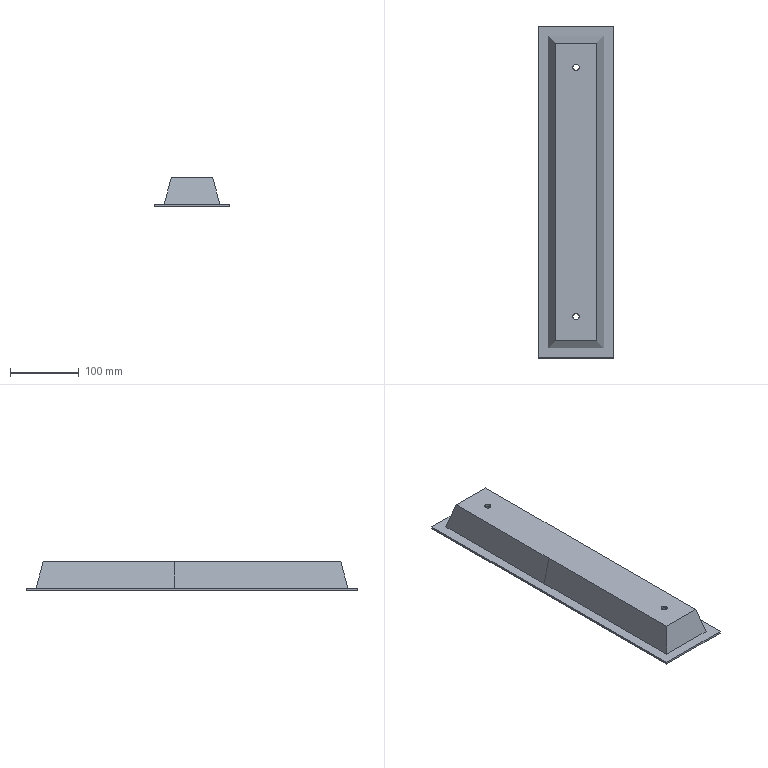Part | NX | features BREP 1 | 1 solid | 28 faces | box 110 x 481.5 x 42.13 mm | volume 250007 mm3 | plane 20 | cylinder 8 | commonest cylinder face diameters 9 x8
STEP:
#1=CARTESIAN_POINT('',(1224.372,-309.5,70.005));
#2=VERTEX_POINT('',#1);
#3=CARTESIAN_POINT('',(1224.372,-309.5,67.005));
#4=VERTEX_POINT('',#3);
#5=CARTESIAN_POINT('',(1224.372,-309.5,68.505));
#6=DIRECTION('',(0.,0.,-1.));
#7=VECTOR('',#6,1000.);
#8=LINE('',#5,#7);
#9=EDGE_CURVE('',#2,#4,#8,.T.);
#10=ORIENTED_EDGE('',*,*,#9,.T.);
#11=CARTESIAN_POINT('',(1224.372,-791.,67.005));
#12=VERTEX_POINT('',#11);
#13=CARTESIAN_POINT('',(1224.372,-550.25,67.005));
#14=DIRECTION('',(0.,1.,0.));
#15=VECTOR('',#14,1000.);
#16=LINE('',#13,#15);
#17=EDGE_CURVE('',#12,#4,#16,.T.);
#18=ORIENTED_EDGE('',*,*,#17,.F.);
#19=CARTESIAN_POINT('',(1224.372,-791.,70.005));
#20=VERTEX_POINT('',#19);
#21=CARTESIAN_POINT('',(1224.372,-791.,68.505));
#22=DIRECTION('',(0.,0.,-1.));
#23=VECTOR('',#22,1000.);
#24=LINE('',#21,#23);
#25=EDGE_CURVE('',#20,#12,#24,.T.);
#26=ORIENTED_EDGE('',*,*,#25,.F.);
#27=CARTESIAN_POINT('',(1224.372,-550.25,70.005));
#28=DIRECTION('',(0.,1.,0.));
#29=VECTOR('',#28,1000.);
#30=LINE('',#27,#29);
#31=EDGE_CURVE('',#20,#2,#30,.T.);
#32=ORIENTED_EDGE('',*,*,#31,.T.);
#33=EDGE_LOOP('',(#10,#18,#26,#32));
#34=FACE_BOUND('',#33,.T.);
#35=CARTESIAN_POINT('',(1224.372,-550.25,70.005));
#36=DIRECTION('',(1.,0.,0.));
#37=DIRECTION('',(0.,0.,-1.));
#38=AXIS2_PLACEMENT_3D('',#35,#36,#37);
#39=PLANE('',#38);
#40=ADVANCED_FACE('',(#34),#39,.F.);
#41=CARTESIAN_POINT('',(1334.372,-791.,70.005));
#42=VERTEX_POINT('',#41);
#43=CARTESIAN_POINT('',(1279.372,-791.,70.005));
#44=DIRECTION('',(1.,0.,0.));
#45=VECTOR('',#44,1000.);
#46=LINE('',#43,#45);
#47=EDGE_CURVE('',#20,#42,#46,.T.);
#48=ORIENTED_EDGE('',*,*,#47,.F.);
#49=ORIENTED_EDGE('',*,*,#25,.T.);
#50=CARTESIAN_POINT('',(1334.372,-791.,67.005));
#51=VERTEX_POINT('',#50);
#52=CARTESIAN_POINT('',(1279.372,-791.,67.005));
#53=DIRECTION('',(1.,0.,0.));
#54=VECTOR('',#53,1000.);
#55=LINE('',#52,#54);
#56=EDGE_CURVE('',#12,#51,#55,.T.);
#57=ORIENTED_EDGE('',*,*,#56,.T.);
#58=CARTESIAN_POINT('',(1334.372,-791.,68.505));
#59=DIRECTION('',(0.,0.,-1.));
#60=VECTOR('',#59,1000.);
#61=LINE('',#58,#60);
#62=EDGE_CURVE('',#42,#51,#61,.T.);
#63=ORIENTED_EDGE('',*,*,#62,.F.);
#64=EDGE_LOOP('',(#48,#49,#57,#63));
#65=FACE_BOUND('',#64,.T.);
#66=CARTESIAN_POINT('',(1279.372,-791.,70.005));
#67=DIRECTION('',(0.,1.,0.));
#68=DIRECTION('',(1.,0.,0.));
#69=AXIS2_PLACEMENT_3D('',#66,#67,#68);
#70=PLANE('',#69);
#71=ADVANCED_FACE('',(#65),#70,.F.);
#72=CARTESIAN_POINT('',(1334.372,-309.5,70.005));
#73=VERTEX_POINT('',#72);
#74=CARTESIAN_POINT('',(1334.372,-550.25,70.005));
#75=DIRECTION('',(0.,-1.,0.));
#76=VECTOR('',#75,1000.);
#77=LINE('',#74,#76);
#78=EDGE_CURVE('',#73,#42,#77,.T.);
#79=ORIENTED_EDGE('',*,*,#78,.T.);
#80=ORIENTED_EDGE('',*,*,#62,.T.);
#81=CARTESIAN_POINT('',(1334.372,-309.5,67.005));
#82=VERTEX_POINT('',#81);
#83=CARTESIAN_POINT('',(1334.372,-550.25,67.005));
#84=DIRECTION('',(0.,1.,0.));
#85=VECTOR('',#84,1000.);
#86=LINE('',#83,#85);
#87=EDGE_CURVE('',#51,#82,#86,.T.);
#88=ORIENTED_EDGE('',*,*,#87,.T.);
#89=CARTESIAN_POINT('',(1334.372,-309.5,68.505));
#90=DIRECTION('',(0.,0.,-1.));
#91=VECTOR('',#90,1000.);
#92=LINE('',#89,#91);
#93=EDGE_CURVE('',#73,#82,#92,.T.);
#94=ORIENTED_EDGE('',*,*,#93,.F.);
#95=EDGE_LOOP('',(#79,#80,#88,#94));
#96=FACE_BOUND('',#95,.T.);
#97=CARTESIAN_POINT('',(1334.372,-550.25,70.005));
#98=DIRECTION('',(-1.,0.,0.));
#99=DIRECTION('',(0.,0.,-1.));
#100=AXIS2_PLACEMENT_3D('',#97,#98,#99);
#101=PLANE('',#100);
#102=ADVANCED_FACE('',(#96),#101,.F.);
#103=CARTESIAN_POINT('',(1279.372,-309.5,70.005));
#104=DIRECTION('',(1.,0.,0.));
#105=VECTOR('',#104,1000.);
#106=LINE('',#103,#105);
#107=EDGE_CURVE('',#2,#73,#106,.T.);
#108=ORIENTED_EDGE('',*,*,#107,.T.);
#109=ORIENTED_EDGE('',*,*,#93,.T.);
#110=CARTESIAN_POINT('',(1279.372,-309.5,67.005));
#111=DIRECTION('',(1.,0.,0.));
#112=VECTOR('',#111,1000.);
#113=LINE('',#110,#112);
#114=EDGE_CURVE('',#4,#82,#113,.T.);
#115=ORIENTED_EDGE('',*,*,#114,.F.);
#116=ORIENTED_EDGE('',*,*,#9,.F.);
#117=EDGE_LOOP('',(#108,#109,#115,#116));
#118=FACE_BOUND('',#117,.T.);
#119=CARTESIAN_POINT('',(1279.372,-309.5,70.005));
#120=DIRECTION('',(0.,1.,0.));
#121=DIRECTION('',(1.,0.,0.));
#122=AXIS2_PLACEMENT_3D('',#119,#120,#121);
#123=PLANE('',#122);
#124=ADVANCED_FACE('',(#118),#123,.T.);
#125=CARTESIAN_POINT('',(1319.857,-776.485,70.005));
#126=VERTEX_POINT('',#125);
#127=CARTESIAN_POINT('',(1319.857,-525.,70.005));
#128=VERTEX_POINT('',#127);
#129=CARTESIAN_POINT('',(1319.857,-776.485,70.005));
#130=CARTESIAN_POINT('',(1319.857,-774.388,70.005));
#131=CARTESIAN_POINT('',(1319.857,-772.291,70.005));
#132=CARTESIAN_POINT('',(1319.857,-770.194,70.005));
#133=CARTESIAN_POINT('',(1319.857,-719.897,70.005));
#134=CARTESIAN_POINT('',(1319.857,-669.6,70.005));
#135=CARTESIAN_POINT('',(1319.857,-621.4,70.005));
#136=CARTESIAN_POINT('',(1319.857,-573.2,70.005));
#137=CARTESIAN_POINT('',(1319.857,-525.,70.005));
#138=B_SPLINE_CURVE_WITH_KNOTS('',5,(#129,#130,#131,#132,#133,#134,#135,#136,#137),.UNSPECIFIED.,.F.,.F.,(6,3,6),(19.538,30.023,271.023),.UNSPECIFIED.);
#139=EDGE_CURVE('',#126,#128,#138,.T.);
#140=ORIENTED_EDGE('',*,*,#139,.F.);
#141=CARTESIAN_POINT('',(1238.887,-776.485,70.005));
#142=VERTEX_POINT('',#141);
#143=CARTESIAN_POINT('',(1238.887,-776.485,70.005));
#144=CARTESIAN_POINT('',(1240.984,-776.485,70.005));
#145=CARTESIAN_POINT('',(1243.081,-776.485,70.005));
#146=CARTESIAN_POINT('',(1245.178,-776.485,70.005));
#147=CARTESIAN_POINT('',(1259.275,-776.485,70.005));
#148=CARTESIAN_POINT('',(1273.372,-776.485,70.005));
#149=CARTESIAN_POINT('',(1285.372,-776.485,70.005));
#150=CARTESIAN_POINT('',(1299.469,-776.485,70.005));
#151=CARTESIAN_POINT('',(1313.566,-776.485,70.005));
#152=CARTESIAN_POINT('',(1315.663,-776.485,70.005));
#153=CARTESIAN_POINT('',(1317.76,-776.485,70.005));
#154=CARTESIAN_POINT('',(1319.857,-776.485,70.005));
#155=B_SPLINE_CURVE_WITH_KNOTS('',5,(#143,#144,#145,#146,#147,#148,#149,#150,#151,#152,#153,#154),.UNSPECIFIED.,.F.,.F.,(6,3,3,6),(19.538,30.023,90.023,100.508),.UNSPECIFIED.);
#156=EDGE_CURVE('',#142,#126,#155,.T.);
#157=ORIENTED_EDGE('',*,*,#156,.F.);
#158=CARTESIAN_POINT('',(1238.887,-525.,70.005));
#159=VERTEX_POINT('',#158);
#160=CARTESIAN_POINT('',(1238.887,-525.,70.005));
#161=CARTESIAN_POINT('',(1238.887,-573.2,70.005));
#162=CARTESIAN_POINT('',(1238.887,-621.4,70.005));
#163=CARTESIAN_POINT('',(1238.887,-669.6,70.005));
#164=CARTESIAN_POINT('',(1238.887,-719.897,70.005));
#165=CARTESIAN_POINT('',(1238.887,-770.194,70.005));
#166=CARTESIAN_POINT('',(1238.887,-772.291,70.005));
#167=CARTESIAN_POINT('',(1238.887,-774.388,70.005));
#168=CARTESIAN_POINT('',(1238.887,-776.485,70.005));
#169=B_SPLINE_CURVE_WITH_KNOTS('',5,(#160,#161,#162,#163,#164,#165,#166,#167,#168),.UNSPECIFIED.,.F.,.F.,(6,3,6),(271.023,512.023,522.508),.UNSPECIFIED.);
#170=EDGE_CURVE('',#159,#142,#169,.T.);
#171=ORIENTED_EDGE('',*,*,#170,.F.);
#172=CARTESIAN_POINT('',(1238.887,-324.015,70.005));
#173=VERTEX_POINT('',#172);
#174=CARTESIAN_POINT('',(1238.887,-324.015,70.005));
#175=CARTESIAN_POINT('',(1238.887,-326.112,70.005));
#176=CARTESIAN_POINT('',(1238.887,-328.209,70.005));
#177=CARTESIAN_POINT('',(1238.887,-330.306,70.005));
#178=CARTESIAN_POINT('',(1238.887,-370.503,70.005));
#179=CARTESIAN_POINT('',(1238.887,-410.7,70.005));
#180=CARTESIAN_POINT('',(1238.887,-448.8,70.005));
#181=CARTESIAN_POINT('',(1238.887,-486.9,70.005));
#182=CARTESIAN_POINT('',(1238.887,-525.,70.005));
#183=B_SPLINE_CURVE_WITH_KNOTS('',5,(#174,#175,#176,#177,#178,#179,#180,#181,#182),.UNSPECIFIED.,.F.,.F.,(6,3,6),(19.538,30.023,220.523),.UNSPECIFIED.);
#184=EDGE_CURVE('',#173,#159,#183,.T.);
#185=ORIENTED_EDGE('',*,*,#184,.F.);
#186=CARTESIAN_POINT('',(1319.857,-324.015,70.005));
#187=VERTEX_POINT('',#186);
#188=CARTESIAN_POINT('',(1319.857,-324.015,70.005));
#189=CARTESIAN_POINT('',(1317.76,-324.015,70.005));
#190=CARTESIAN_POINT('',(1315.663,-324.015,70.005));
#191=CARTESIAN_POINT('',(1313.566,-324.015,70.005));
#192=CARTESIAN_POINT('',(1299.469,-324.015,70.005));
#193=CARTESIAN_POINT('',(1285.372,-324.015,70.005));
#194=CARTESIAN_POINT('',(1273.372,-324.015,70.005));
#195=CARTESIAN_POINT('',(1259.275,-324.015,70.005));
#196=CARTESIAN_POINT('',(1245.178,-324.015,70.005));
#197=CARTESIAN_POINT('',(1243.081,-324.015,70.005));
#198=CARTESIAN_POINT('',(1240.984,-324.015,70.005));
#199=CARTESIAN_POINT('',(1238.887,-324.015,70.005));
#200=B_SPLINE_CURVE_WITH_KNOTS('',5,(#188,#189,#190,#191,#192,#193,#194,#195,#196,#197,#198,#199),.UNSPECIFIED.,.F.,.F.,(6,3,3,6),(19.538,30.023,90.023,100.508),.UNSPECIFIED.);
#201=EDGE_CURVE('',#187,#173,#200,.T.);
#202=ORIENTED_EDGE('',*,*,#201,.F.);
#203=CARTESIAN_POINT('',(1319.857,-525.,70.005));
#204=CARTESIAN_POINT('',(1319.857,-486.9,70.005));
#205=CARTESIAN_POINT('',(1319.857,-448.8,70.005));
#206=CARTESIAN_POINT('',(1319.857,-410.7,70.005));
#207=CARTESIAN_POINT('',(1319.857,-370.503,70.005));
#208=CARTESIAN_POINT('',(1319.857,-330.306,70.005));
#209=CARTESIAN_POINT('',(1319.857,-328.209,70.005));
#210=CARTESIAN_POINT('',(1319.857,-326.112,70.005));
#211=CARTESIAN_POINT('',(1319.857,-324.015,70.005));
#212=B_SPLINE_CURVE_WITH_KNOTS('',5,(#203,#204,#205,#206,#207,#208,#209,#210,#211),.UNSPECIFIED.,.F.,.F.,(6,3,6),(321.523,512.023,522.508),.UNSPECIFIED.);
#213=EDGE_CURVE('',#128,#187,#212,.T.);
#214=ORIENTED_EDGE('',*,*,#213,.F.);
#215=EDGE_LOOP('',(#140,#157,#171,#185,#202,#214));
#216=FACE_BOUND('',#215,.T.);
#217=ORIENTED_EDGE('',*,*,#31,.F.);
#218=ORIENTED_EDGE('',*,*,#47,.T.);
#219=ORIENTED_EDGE('',*,*,#78,.F.);
#220=ORIENTED_EDGE('',*,*,#107,.F.);
#221=EDGE_LOOP('',(#217,#218,#219,#220));
#222=FACE_BOUND('',#221,.T.);
#223=CARTESIAN_POINT('',(0.,-525.,70.005));
#224=DIRECTION('',(0.,0.,1.));
#225=DIRECTION('',(1.,0.,0.));
#226=AXIS2_PLACEMENT_3D('',#223,#224,#225);
#227=PLANE('',#226);
#228=ADVANCED_FACE('',(#216,#222),#227,.T.);
#229=CARTESIAN_POINT('',(1317.555,-525.,67.005));
#230=VERTEX_POINT('',#229);
#231=CARTESIAN_POINT('',(1317.555,-326.317,67.005));
#232=VERTEX_POINT('',#231);
#233=CARTESIAN_POINT('',(1317.555,-525.,67.005));
#234=CARTESIAN_POINT('',(1317.555,-485.263,67.005));
#235=CARTESIAN_POINT('',(1317.555,-445.527,67.005));
#236=CARTESIAN_POINT('',(1317.555,-405.79,67.005));
#237=CARTESIAN_POINT('',(1317.555,-366.054,67.005));
#238=CARTESIAN_POINT('',(1317.555,-326.317,67.005));
#239=B_SPLINE_CURVE_WITH_KNOTS('',5,(#233,#234,#235,#236,#237,#238),.UNSPECIFIED.,.F.,.F.,(6,6),(321.523,520.206),.UNSPECIFIED.);
#240=EDGE_CURVE('',#230,#232,#239,.T.);
#241=ORIENTED_EDGE('',*,*,#240,.T.);
#242=CARTESIAN_POINT('',(1241.189,-326.317,67.005));
#243=VERTEX_POINT('',#242);
#244=CARTESIAN_POINT('',(1317.555,-326.317,67.005));
#245=CARTESIAN_POINT('',(1302.282,-326.317,67.005));
#246=CARTESIAN_POINT('',(1287.009,-326.317,67.005));
#247=CARTESIAN_POINT('',(1271.736,-326.317,67.005));
#248=CARTESIAN_POINT('',(1256.463,-326.317,67.005));
#249=CARTESIAN_POINT('',(1241.189,-326.317,67.005));
#250=B_SPLINE_CURVE_WITH_KNOTS('',5,(#244,#245,#246,#247,#248,#249),.UNSPECIFIED.,.F.,.F.,(6,6),(21.84,98.206),.UNSPECIFIED.);
#251=EDGE_CURVE('',#232,#243,#250,.T.);
#252=ORIENTED_EDGE('',*,*,#251,.T.);
#253=CARTESIAN_POINT('',(1241.189,-525.,67.005));
#254=VERTEX_POINT('',#253);
#255=CARTESIAN_POINT('',(1241.189,-326.317,67.005));
#256=CARTESIAN_POINT('',(1241.189,-366.054,67.005));
#257=CARTESIAN_POINT('',(1241.189,-405.79,67.005));
#258=CARTESIAN_POINT('',(1241.189,-445.527,67.005));
#259=CARTESIAN_POINT('',(1241.189,-485.263,67.005));
#260=CARTESIAN_POINT('',(1241.189,-525.,67.005));
#261=B_SPLINE_CURVE_WITH_KNOTS('',5,(#255,#256,#257,#258,#259,#260),.UNSPECIFIED.,.F.,.F.,(6,6),(21.84,220.523),.UNSPECIFIED.);
#262=EDGE_CURVE('',#243,#254,#261,.T.);
#263=ORIENTED_EDGE('',*,*,#262,.T.);
#264=CARTESIAN_POINT('',(1241.189,-774.183,67.005));
#265=VERTEX_POINT('',#264);
#266=CARTESIAN_POINT('',(1241.189,-525.,67.005));
#267=CARTESIAN_POINT('',(1241.189,-574.837,67.005));
#268=CARTESIAN_POINT('',(1241.189,-624.673,67.005));
#269=CARTESIAN_POINT('',(1241.189,-674.51,67.005));
#270=CARTESIAN_POINT('',(1241.189,-724.346,67.005));
#271=CARTESIAN_POINT('',(1241.189,-774.183,67.005));
#272=B_SPLINE_CURVE_WITH_KNOTS('',5,(#266,#267,#268,#269,#270,#271),.UNSPECIFIED.,.F.,.F.,(6,6),(271.023,520.206),.UNSPECIFIED.);
#273=EDGE_CURVE('',#254,#265,#272,.T.);
#274=ORIENTED_EDGE('',*,*,#273,.T.);
#275=CARTESIAN_POINT('',(1317.555,-774.183,67.005));
#276=VERTEX_POINT('',#275);
#277=CARTESIAN_POINT('',(1279.372,-774.183,67.005));
#278=DIRECTION('',(1.,0.,0.));
#279=VECTOR('',#278,1000.);
#280=LINE('',#277,#279);
#281=EDGE_CURVE('',#265,#276,#280,.T.);
#282=ORIENTED_EDGE('',*,*,#281,.T.);
#283=CARTESIAN_POINT('',(1317.555,-774.183,67.005));
#284=CARTESIAN_POINT('',(1317.555,-724.346,67.005));
#285=CARTESIAN_POINT('',(1317.555,-674.51,67.005));
#286=CARTESIAN_POINT('',(1317.555,-624.673,67.005));
#287=CARTESIAN_POINT('',(1317.555,-574.837,67.005));
#288=CARTESIAN_POINT('',(1317.555,-525.,67.005));
#289=B_SPLINE_CURVE_WITH_KNOTS('',5,(#283,#284,#285,#286,#287,#288),.UNSPECIFIED.,.F.,.F.,(6,6),(21.84,271.023),.UNSPECIFIED.);
#290=EDGE_CURVE('',#276,#230,#289,.T.);
#291=ORIENTED_EDGE('',*,*,#290,.T.);
#292=EDGE_LOOP('',(#241,#252,#263,#274,#282,#291));
#293=FACE_BOUND('',#292,.T.);
#294=ORIENTED_EDGE('',*,*,#114,.T.);
#295=ORIENTED_EDGE('',*,*,#87,.F.);
#296=ORIENTED_EDGE('',*,*,#56,.F.);
#297=ORIENTED_EDGE('',*,*,#17,.T.);
#298=EDGE_LOOP('',(#294,#295,#296,#297));
#299=FACE_BOUND('',#298,.T.);
#300=CARTESIAN_POINT('',(0.,-525.,67.005));
#301=DIRECTION('',(0.,0.,1.));
#302=DIRECTION('',(1.,0.,0.));
#303=AXIS2_PLACEMENT_3D('',#300,#301,#302);
#304=PLANE('',#303);
#305=ADVANCED_FACE('',(#293,#299),#304,.F.);
#306=CARTESIAN_POINT('',(1249.372,-525.,109.135));
#307=VERTEX_POINT('',#306);
#308=CARTESIAN_POINT('',(1238.887,-525.,70.005));
#309=CARTESIAN_POINT('',(1249.372,-525.,109.135));
#310=B_SPLINE_CURVE_WITH_KNOTS('',1,(#308,#309),.UNSPECIFIED.,.F.,.F.,(2,2),(17.49,58.),.UNSPECIFIED.);
#311=EDGE_CURVE('',#159,#307,#310,.T.);
#312=ORIENTED_EDGE('',*,*,#311,.F.);
#313=ORIENTED_EDGE('',*,*,#170,.T.);
#314=CARTESIAN_POINT('',(1249.372,-766.,109.135));
#315=VERTEX_POINT('',#314);
#316=CARTESIAN_POINT('',(1238.887,-776.485,70.005));
#317=CARTESIAN_POINT('',(1249.372,-766.,109.135));
#318=B_SPLINE_CURVE_WITH_KNOTS('',1,(#316,#317),.UNSPECIFIED.,.F.,.F.,(2,2),(-20.923,20.923),.UNSPECIFIED.);
#319=EDGE_CURVE('',#142,#315,#318,.T.);
#320=ORIENTED_EDGE('',*,*,#319,.T.);
#321=CARTESIAN_POINT('',(1249.372,-645.5,109.135));
#322=DIRECTION('',(0.,-1.,0.));
#323=VECTOR('',#322,1000.);
#324=LINE('',#321,#323);
#325=EDGE_CURVE('',#307,#315,#324,.T.);
#326=ORIENTED_EDGE('',*,*,#325,.F.);
#327=EDGE_LOOP('',(#312,#313,#320,#326));
#328=FACE_BOUND('',#327,.T.);
#329=CARTESIAN_POINT('',(1241.866,-525.,81.123));
#330=DIRECTION('',(-0.9659,0.,0.2588));
#331=DIRECTION('',(0.2588,0.,0.9659));
#332=AXIS2_PLACEMENT_3D('',#329,#330,#331);
#333=PLANE('',#332);
#334=ADVANCED_FACE('',(#328),#333,.T.);
#335=ORIENTED_EDGE('',*,*,#311,.T.);
#336=CARTESIAN_POINT('',(1249.372,-334.5,109.135));
#337=VERTEX_POINT('',#336);
#338=CARTESIAN_POINT('',(1249.372,-429.75,109.135));
#339=DIRECTION('',(0.,-1.,0.));
#340=VECTOR('',#339,1000.);
#341=LINE('',#338,#340);
#342=EDGE_CURVE('',#337,#307,#341,.T.);
#343=ORIENTED_EDGE('',*,*,#342,.F.);
#344=CARTESIAN_POINT('',(1238.887,-324.015,70.005));
#345=CARTESIAN_POINT('',(1242.382,-327.51,83.048));
#346=CARTESIAN_POINT('',(1245.877,-331.005,96.091));
#347=CARTESIAN_POINT('',(1249.372,-334.5,109.135));
#348=B_SPLINE_CURVE_WITH_KNOTS('',3,(#344,#345,#346,#347),.UNSPECIFIED.,.F.,.F.,(4,4),(-20.923,20.923),.UNSPECIFIED.);
#349=EDGE_CURVE('',#173,#337,#348,.T.);
#350=ORIENTED_EDGE('',*,*,#349,.F.);
#351=ORIENTED_EDGE('',*,*,#184,.T.);
#352=EDGE_LOOP('',(#335,#343,#350,#351));
#353=FACE_BOUND('',#352,.T.);
#354=CARTESIAN_POINT('',(1241.866,-575.5,81.123));
#355=DIRECTION('',(-0.9659,0.,0.2588));
#356=DIRECTION('',(0.2588,0.,0.9659));
#357=AXIS2_PLACEMENT_3D('',#354,#355,#356);
#358=PLANE('',#357);
#359=ADVANCED_FACE('',(#353),#358,.T.);
#360=CARTESIAN_POINT('',(1309.372,-334.5,109.135));
#361=VERTEX_POINT('',#360);
#362=CARTESIAN_POINT('',(1279.372,-334.5,109.135));
#363=DIRECTION('',(-1.,0.,0.));
#364=VECTOR('',#363,1000.);
#365=LINE('',#362,#364);
#366=EDGE_CURVE('',#361,#337,#365,.T.);
#367=ORIENTED_EDGE('',*,*,#366,.F.);
#368=CARTESIAN_POINT('',(1319.857,-324.015,70.005));
#369=CARTESIAN_POINT('',(1309.372,-334.5,109.135));
#370=B_SPLINE_CURVE_WITH_KNOTS('',1,(#368,#369),.UNSPECIFIED.,.F.,.F.,(2,2),(-20.923,20.923),.UNSPECIFIED.);
#371=EDGE_CURVE('',#187,#361,#370,.T.);
#372=ORIENTED_EDGE('',*,*,#371,.F.);
#373=ORIENTED_EDGE('',*,*,#201,.T.);
#374=ORIENTED_EDGE('',*,*,#349,.T.);
#375=EDGE_LOOP('',(#367,#372,#373,#374));
#376=FACE_BOUND('',#375,.T.);
#377=CARTESIAN_POINT('',(1279.372,-326.994,81.123));
#378=DIRECTION('',(0.,0.9659,0.2588));
#379=DIRECTION('',(0.,-0.2588,0.9659));
#380=AXIS2_PLACEMENT_3D('',#377,#378,#379);
#381=PLANE('',#380);
#382=ADVANCED_FACE('',(#376),#381,.T.);
#383=CARTESIAN_POINT('',(1309.372,-525.,109.135));
#384=VERTEX_POINT('',#383);
#385=CARTESIAN_POINT('',(1319.857,-525.,70.005));
#386=CARTESIAN_POINT('',(1309.372,-525.,109.135));
#387=B_SPLINE_CURVE_WITH_KNOTS('',1,(#385,#386),.UNSPECIFIED.,.F.,.F.,(2,2),(17.49,58.),.UNSPECIFIED.);
#388=EDGE_CURVE('',#128,#384,#387,.T.);
#389=ORIENTED_EDGE('',*,*,#388,.F.);
#390=ORIENTED_EDGE('',*,*,#213,.T.);
#391=ORIENTED_EDGE('',*,*,#371,.T.);
#392=CARTESIAN_POINT('',(1309.372,-429.75,109.135));
#393=DIRECTION('',(0.,1.,0.));
#394=VECTOR('',#393,1000.);
#395=LINE('',#392,#394);
#396=EDGE_CURVE('',#384,#361,#395,.T.);
#397=ORIENTED_EDGE('',*,*,#396,.F.);
#398=EDGE_LOOP('',(#389,#390,#391,#397));
#399=FACE_BOUND('',#398,.T.);
#400=CARTESIAN_POINT('',(1316.878,-575.5,81.123));
#401=DIRECTION('',(0.9659,0.,0.2588));
#402=DIRECTION('',(0.2588,0.,-0.9659));
#403=AXIS2_PLACEMENT_3D('',#400,#401,#402);
#404=PLANE('',#403);
#405=ADVANCED_FACE('',(#399),#404,.T.);
#406=CARTESIAN_POINT('',(1309.372,-766.,109.135));
#407=VERTEX_POINT('',#406);
#408=CARTESIAN_POINT('',(1309.372,-645.5,109.135));
#409=DIRECTION('',(0.,1.,0.));
#410=VECTOR('',#409,1000.);
#411=LINE('',#408,#410);
#412=EDGE_CURVE('',#407,#384,#411,.T.);
#413=ORIENTED_EDGE('',*,*,#412,.F.);
#414=CARTESIAN_POINT('',(1319.857,-776.485,70.005));
#415=CARTESIAN_POINT('',(1309.372,-766.,109.135));
#416=B_SPLINE_CURVE_WITH_KNOTS('',1,(#414,#415),.UNSPECIFIED.,.F.,.F.,(2,2),(-20.923,20.923),.UNSPECIFIED.);
#417=EDGE_CURVE('',#126,#407,#416,.T.);
#418=ORIENTED_EDGE('',*,*,#417,.F.);
#419=ORIENTED_EDGE('',*,*,#139,.T.);
#420=ORIENTED_EDGE('',*,*,#388,.T.);
#421=EDGE_LOOP('',(#413,#418,#419,#420));
#422=FACE_BOUND('',#421,.T.);
#423=CARTESIAN_POINT('',(1316.878,-525.,81.123));
#424=DIRECTION('',(0.9659,0.,0.2588));
#425=DIRECTION('',(0.2588,0.,-0.9659));
#426=AXIS2_PLACEMENT_3D('',#423,#424,#425);
#427=PLANE('',#426);
#428=ADVANCED_FACE('',(#422),#427,.T.);
#429=CARTESIAN_POINT('',(1279.372,-766.,109.135));
#430=DIRECTION('',(1.,0.,0.));
#431=VECTOR('',#430,1000.);
#432=LINE('',#429,#431);
#433=EDGE_CURVE('',#315,#407,#432,.T.);
#434=ORIENTED_EDGE('',*,*,#433,.F.);
#435=ORIENTED_EDGE('',*,*,#319,.F.);
#436=ORIENTED_EDGE('',*,*,#156,.T.);
#437=ORIENTED_EDGE('',*,*,#417,.T.);
#438=EDGE_LOOP('',(#434,#435,#436,#437));
#439=FACE_BOUND('',#438,.T.);
#440=CARTESIAN_POINT('',(1279.372,-773.506,81.123));
#441=DIRECTION('',(0.,-0.9659,0.2588));
#442=DIRECTION('',(0.,-0.2588,-0.9659));
#443=AXIS2_PLACEMENT_3D('',#440,#441,#442);
#444=PLANE('',#443);
#445=ADVANCED_FACE('',(#439),#444,.T.);
#446=CARTESIAN_POINT('',(1274.872,-731.,106.135));
#447=VERTEX_POINT('',#446);
#448=CARTESIAN_POINT('',(1279.372,-735.5,106.135));
#449=VERTEX_POINT('',#448);
#450=CARTESIAN_POINT('',(1279.372,-731.,106.135));
#451=DIRECTION('',(0.,0.,1.));
#452=DIRECTION('',(1.,0.,0.));
#453=AXIS2_PLACEMENT_3D('',#450,#451,#452);
#454=CIRCLE('',#453,4.5);
#455=EDGE_CURVE('',#447,#449,#454,.T.);
#456=ORIENTED_EDGE('',*,*,#455,.F.);
#457=CARTESIAN_POINT('',(1274.872,-731.,109.135));
#458=VERTEX_POINT('',#457);
#459=CARTESIAN_POINT('',(1274.872,-731.,109.135));
#460=DIRECTION('',(0.,0.,1.));
#461=VECTOR('',#460,1000.);
#462=LINE('',#459,#461);
#463=EDGE_CURVE('',#447,#458,#462,.T.);
#464=ORIENTED_EDGE('',*,*,#463,.T.);
#465=CARTESIAN_POINT('',(1279.372,-735.5,109.135));
#466=VERTEX_POINT('',#465);
#467=CARTESIAN_POINT('',(1279.372,-731.,109.135));
#468=DIRECTION('',(0.,0.,1.));
#469=DIRECTION('',(1.,0.,0.));
#470=AXIS2_PLACEMENT_3D('',#467,#468,#469);
#471=CIRCLE('',#470,4.5);
#472=EDGE_CURVE('',#458,#466,#471,.T.);
#473=ORIENTED_EDGE('',*,*,#472,.T.);
#474=CARTESIAN_POINT('',(1279.372,-735.5,109.135));
#475=DIRECTION('',(0.,0.,1.));
#476=VECTOR('',#475,1000.);
#477=LINE('',#474,#476);
#478=EDGE_CURVE('',#449,#466,#477,.T.);
#479=ORIENTED_EDGE('',*,*,#478,.F.);
#480=EDGE_LOOP('',(#456,#464,#473,#479));
#481=FACE_BOUND('',#480,.T.);
#482=CARTESIAN_POINT('',(1279.372,-731.,109.135));
#483=DIRECTION('',(0.,0.,1.));
#484=DIRECTION('',(0.,1.,0.));
#485=AXIS2_PLACEMENT_3D('',#482,#483,#484);
#486=CYLINDRICAL_SURFACE('',#485,4.5);
#487=ADVANCED_FACE('',(#481),#486,.F.);
#488=CARTESIAN_POINT('',(1279.372,-365.,109.135));
#489=VERTEX_POINT('',#488);
#490=CARTESIAN_POINT('',(1274.872,-369.5,109.135));
#491=VERTEX_POINT('',#490);
#492=CARTESIAN_POINT('',(1279.372,-369.5,109.135));
#493=DIRECTION('',(0.,0.,1.));
#494=DIRECTION('',(1.,0.,0.));
#495=AXIS2_PLACEMENT_3D('',#492,#493,#494);
#496=CIRCLE('',#495,4.5);
#497=EDGE_CURVE('',#489,#491,#496,.T.);
#498=ORIENTED_EDGE('',*,*,#497,.T.);
#499=CARTESIAN_POINT('',(1274.872,-369.5,106.135));
#500=VERTEX_POINT('',#499);
#501=CARTESIAN_POINT('',(1274.872,-369.5,109.135));
#502=DIRECTION('',(0.,0.,1.));
#503=VECTOR('',#502,1000.);
#504=LINE('',#501,#503);
#505=EDGE_CURVE('',#500,#491,#504,.T.);
#506=ORIENTED_EDGE('',*,*,#505,.F.);
#507=CARTESIAN_POINT('',(1279.372,-365.,106.135));
#508=VERTEX_POINT('',#507);
#509=CARTESIAN_POINT('',(1279.372,-365.,106.135));
#510=CARTESIAN_POINT('',(1278.191,-365.,106.135));
#511=CARTESIAN_POINT('',(1275.849,-365.977,106.135));
#512=CARTESIAN_POINT('',(1274.872,-368.317,106.135));
#513=CARTESIAN_POINT('',(1274.872,-369.5,106.135));
#514=B_SPLINE_CURVE_WITH_KNOTS('',3,(#509,#510,#511,#512,#513),.UNSPECIFIED.,.F.,.F.,(4,1,4),(0.,0.5,1.),.UNSPECIFIED.);
#515=EDGE_CURVE('',#508,#500,#514,.T.);
#516=ORIENTED_EDGE('',*,*,#515,.F.);
#517=CARTESIAN_POINT('',(1279.372,-365.,109.135));
#518=DIRECTION('',(0.,0.,1.));
#519=VECTOR('',#518,1000.);
#520=LINE('',#517,#519);
#521=EDGE_CURVE('',#508,#489,#520,.T.);
#522=ORIENTED_EDGE('',*,*,#521,.T.);
#523=EDGE_LOOP('',(#498,#506,#516,#522));
#524=FACE_BOUND('',#523,.T.);
#525=CARTESIAN_POINT('',(1279.372,-369.5,109.135));
#526=DIRECTION('',(0.,0.,1.));
#527=DIRECTION('',(0.,1.,0.));
#528=AXIS2_PLACEMENT_3D('',#525,#526,#527);
#529=CYLINDRICAL_SURFACE('',#528,4.5);
#530=ADVANCED_FACE('',(#524),#529,.F.);
#531=CARTESIAN_POINT('',(1283.872,-369.5,106.135));
#532=VERTEX_POINT('',#531);
#533=CARTESIAN_POINT('',(1283.872,-369.5,106.135));
#534=CARTESIAN_POINT('',(1283.872,-368.319,106.135));
#535=CARTESIAN_POINT('',(1282.895,-365.977,106.135));
#536=CARTESIAN_POINT('',(1280.555,-365.,106.135));
#537=CARTESIAN_POINT('',(1279.372,-365.,106.135));
#538=B_SPLINE_CURVE_WITH_KNOTS('',3,(#533,#534,#535,#536,#537),.UNSPECIFIED.,.F.,.F.,(4,1,4),(0.,0.5,1.),.UNSPECIFIED.);
#539=EDGE_CURVE('',#532,#508,#538,.T.);
#540=ORIENTED_EDGE('',*,*,#539,.F.);
#541=CARTESIAN_POINT('',(1283.872,-369.5,109.135));
#542=VERTEX_POINT('',#541);
#543=CARTESIAN_POINT('',(1283.872,-369.5,109.135));
#544=DIRECTION('',(0.,0.,1.));
#545=VECTOR('',#544,1000.);
#546=LINE('',#543,#545);
#547=EDGE_CURVE('',#532,#542,#546,.T.);
#548=ORIENTED_EDGE('',*,*,#547,.T.);
#549=CARTESIAN_POINT('',(1279.372,-369.5,109.135));
#550=DIRECTION('',(0.,0.,1.));
#551=DIRECTION('',(1.,0.,0.));
#552=AXIS2_PLACEMENT_3D('',#549,#550,#551);
#553=CIRCLE('',#552,4.5);
#554=EDGE_CURVE('',#542,#489,#553,.T.);
#555=ORIENTED_EDGE('',*,*,#554,.T.);
#556=ORIENTED_EDGE('',*,*,#521,.F.);
#557=EDGE_LOOP('',(#540,#548,#555,#556));
#558=FACE_BOUND('',#557,.T.);
#559=CARTESIAN_POINT('',(1279.372,-369.5,109.135));
#560=DIRECTION('',(0.,0.,1.));
#561=DIRECTION('',(0.,-1.,0.));
#562=AXIS2_PLACEMENT_3D('',#559,#560,#561);
#563=CYLINDRICAL_SURFACE('',#562,4.5);
#564=ADVANCED_FACE('',(#558),#563,.F.);
#565=CARTESIAN_POINT('',(1279.372,-374.,109.135));
#566=VERTEX_POINT('',#565);
#567=CARTESIAN_POINT('',(1279.372,-369.5,109.135));
#568=DIRECTION('',(0.,0.,1.));
#569=DIRECTION('',(1.,0.,0.));
#570=AXIS2_PLACEMENT_3D('',#567,#568,#569);
#571=CIRCLE('',#570,4.5);
#572=EDGE_CURVE('',#566,#542,#571,.T.);
#573=ORIENTED_EDGE('',*,*,#572,.T.);
#574=ORIENTED_EDGE('',*,*,#547,.F.);
#575=CARTESIAN_POINT('',(1279.372,-374.,106.135));
#576=VERTEX_POINT('',#575);
#577=CARTESIAN_POINT('',(1279.372,-374.,106.135));
#578=CARTESIAN_POINT('',(1280.553,-374.,106.135));
#579=CARTESIAN_POINT('',(1282.896,-373.023,106.135));
#580=CARTESIAN_POINT('',(1283.872,-370.683,106.135));
#581=CARTESIAN_POINT('',(1283.872,-369.5,106.135));
#582=B_SPLINE_CURVE_WITH_KNOTS('',3,(#577,#578,#579,#580,#581),.UNSPECIFIED.,.F.,.F.,(4,1,4),(0.,0.5,1.),.UNSPECIFIED.);
#583=EDGE_CURVE('',#576,#532,#582,.T.);
#584=ORIENTED_EDGE('',*,*,#583,.F.);
#585=CARTESIAN_POINT('',(1279.372,-374.,109.135));
#586=DIRECTION('',(0.,0.,1.));
#587=VECTOR('',#586,1000.);
#588=LINE('',#585,#587);
#589=EDGE_CURVE('',#576,#566,#588,.T.);
#590=ORIENTED_EDGE('',*,*,#589,.T.);
#591=EDGE_LOOP('',(#573,#574,#584,#590));
#592=FACE_BOUND('',#591,.T.);
#593=CARTESIAN_POINT('',(1279.372,-369.5,109.135));
#594=DIRECTION('',(0.,0.,1.));
#595=DIRECTION('',(0.,-1.,0.));
#596=AXIS2_PLACEMENT_3D('',#593,#594,#595);
#597=CYLINDRICAL_SURFACE('',#596,4.5);
#598=ADVANCED_FACE('',(#592),#597,.F.);
#599=CARTESIAN_POINT('',(1274.872,-369.5,106.135));
#600=CARTESIAN_POINT('',(1274.872,-370.681,106.135));
#601=CARTESIAN_POINT('',(1275.85,-373.023,106.135));
#602=CARTESIAN_POINT('',(1278.19,-374.,106.135));
#603=CARTESIAN_POINT('',(1279.372,-374.,106.135));
#604=B_SPLINE_CURVE_WITH_KNOTS('',3,(#599,#600,#601,#602,#603),.UNSPECIFIED.,.F.,.F.,(4,1,4),(0.,0.5,1.),.UNSPECIFIED.);
#605=EDGE_CURVE('',#500,#576,#604,.T.);
#606=ORIENTED_EDGE('',*,*,#605,.F.);
#607=ORIENTED_EDGE('',*,*,#505,.T.);
#608=CARTESIAN_POINT('',(1279.372,-369.5,109.135));
#609=DIRECTION('',(0.,0.,1.));
#610=DIRECTION('',(1.,0.,0.));
#611=AXIS2_PLACEMENT_3D('',#608,#609,#610);
#612=CIRCLE('',#611,4.5);
#613=EDGE_CURVE('',#491,#566,#612,.T.);
#614=ORIENTED_EDGE('',*,*,#613,.T.);
#615=ORIENTED_EDGE('',*,*,#589,.F.);
#616=EDGE_LOOP('',(#606,#607,#614,#615));
#617=FACE_BOUND('',#616,.T.);
#618=CARTESIAN_POINT('',(1279.372,-369.5,109.135));
#619=DIRECTION('',(0.,0.,1.));
#620=DIRECTION('',(0.,1.,0.));
#621=AXIS2_PLACEMENT_3D('',#618,#619,#620);
#622=CYLINDRICAL_SURFACE('',#621,4.5);
#623=ADVANCED_FACE('',(#617),#622,.F.);
#624=CARTESIAN_POINT('',(1307.07,-763.698,106.135));
#625=VERTEX_POINT('',#624);
#626=CARTESIAN_POINT('',(1317.555,-774.183,67.005));
#627=CARTESIAN_POINT('',(1307.07,-763.698,106.135));
#628=B_SPLINE_CURVE_WITH_KNOTS('',1,(#626,#627),.UNSPECIFIED.,.F.,.F.,(2,2),(-20.923,20.923),.UNSPECIFIED.);
#629=EDGE_CURVE('',#276,#625,#628,.T.);
#630=ORIENTED_EDGE('',*,*,#629,.F.);
#631=ORIENTED_EDGE('',*,*,#281,.F.);
#632=CARTESIAN_POINT('',(1251.674,-763.698,106.135));
#633=VERTEX_POINT('',#632);
#634=CARTESIAN_POINT('',(1241.189,-774.183,67.005));
#635=CARTESIAN_POINT('',(1251.674,-763.698,106.135));
#636=B_SPLINE_CURVE_WITH_KNOTS('',1,(#634,#635),.UNSPECIFIED.,.F.,.F.,(2,2),(-20.923,20.923),.UNSPECIFIED.);
#637=EDGE_CURVE('',#265,#633,#636,.T.);
#638=ORIENTED_EDGE('',*,*,#637,.T.);
#639=CARTESIAN_POINT('',(1279.372,-763.698,106.135));
#640=DIRECTION('',(1.,0.,0.));
#641=VECTOR('',#640,1000.);
#642=LINE('',#639,#641);
#643=EDGE_CURVE('',#633,#625,#642,.T.);
#644=ORIENTED_EDGE('',*,*,#643,.T.);
#645=EDGE_LOOP('',(#630,#631,#638,#644));
#646=FACE_BOUND('',#645,.T.);
#647=CARTESIAN_POINT('',(1241.189,-774.183,67.005));
#648=DIRECTION('',(0.,-0.9659,0.2588));
#649=DIRECTION('',(1.,0.,0.));
#650=AXIS2_PLACEMENT_3D('',#647,#648,#649);
#651=PLANE('',#650);
#652=ADVANCED_FACE('',(#646),#651,.F.);
#653=CARTESIAN_POINT('',(1307.07,-525.,106.135));
#654=VERTEX_POINT('',#653);
#655=CARTESIAN_POINT('',(1317.555,-525.,67.005));
#656=CARTESIAN_POINT('',(1307.07,-525.,106.135));
#657=B_SPLINE_CURVE_WITH_KNOTS('',1,(#655,#656),.UNSPECIFIED.,.F.,.F.,(2,2),(15.188,55.698),.UNSPECIFIED.);
#658=EDGE_CURVE('',#230,#654,#657,.T.);
#659=ORIENTED_EDGE('',*,*,#658,.F.);
#660=ORIENTED_EDGE('',*,*,#290,.F.);
#661=ORIENTED_EDGE('',*,*,#629,.T.);
#662=CARTESIAN_POINT('',(1307.07,-644.349,106.135));
#663=DIRECTION('',(0.,1.,0.));
#664=VECTOR('',#663,1000.);
#665=LINE('',#662,#664);
#666=EDGE_CURVE('',#625,#654,#665,.T.);
#667=ORIENTED_EDGE('',*,*,#666,.T.);
#668=EDGE_LOOP('',(#659,#660,#661,#667));
#669=FACE_BOUND('',#668,.T.);
#670=CARTESIAN_POINT('',(1312.313,-649.591,86.57));
#671=DIRECTION('',(0.9659,0.,0.2588));
#672=DIRECTION('',(0.2588,0.,-0.9659));
#673=AXIS2_PLACEMENT_3D('',#670,#671,#672);
#674=PLANE('',#673);
#675=ADVANCED_FACE('',(#669),#674,.F.);
#676=CARTESIAN_POINT('',(1307.07,-336.802,106.135));
#677=VERTEX_POINT('',#676);
#678=CARTESIAN_POINT('',(1307.07,-430.901,106.135));
#679=DIRECTION('',(0.,1.,0.));
#680=VECTOR('',#679,1000.);
#681=LINE('',#678,#680);
#682=EDGE_CURVE('',#654,#677,#681,.T.);
#683=ORIENTED_EDGE('',*,*,#682,.T.);
#684=CARTESIAN_POINT('',(1317.555,-326.317,67.005));
#685=CARTESIAN_POINT('',(1312.313,-331.56,86.57));
#686=CARTESIAN_POINT('',(1307.07,-336.802,106.135));
#687=B_SPLINE_CURVE_WITH_KNOTS('',2,(#684,#685,#686),.UNSPECIFIED.,.F.,.F.,(3,3),(-20.923,20.923),.UNSPECIFIED.);
#688=EDGE_CURVE('',#232,#677,#687,.T.);
#689=ORIENTED_EDGE('',*,*,#688,.F.);
#690=ORIENTED_EDGE('',*,*,#240,.F.);
#691=ORIENTED_EDGE('',*,*,#658,.T.);
#692=EDGE_LOOP('',(#683,#689,#690,#691));
#693=FACE_BOUND('',#692,.T.);
#694=CARTESIAN_POINT('',(1312.313,-425.659,86.57));
#695=DIRECTION('',(0.9659,0.,0.2588));
#696=DIRECTION('',(0.2588,0.,-0.9659));
#697=AXIS2_PLACEMENT_3D('',#694,#695,#696);
#698=PLANE('',#697);
#699=ADVANCED_FACE('',(#693),#698,.F.);
#700=CARTESIAN_POINT('',(1251.674,-336.802,106.135));
#701=VERTEX_POINT('',#700);
#702=CARTESIAN_POINT('',(1241.189,-326.317,67.005));
#703=CARTESIAN_POINT('',(1251.674,-336.802,106.135));
#704=B_SPLINE_CURVE_WITH_KNOTS('',1,(#702,#703),.UNSPECIFIED.,.F.,.F.,(2,2),(-20.923,20.923),.UNSPECIFIED.);
#705=EDGE_CURVE('',#243,#701,#704,.T.);
#706=ORIENTED_EDGE('',*,*,#705,.F.);
#707=ORIENTED_EDGE('',*,*,#251,.F.);
#708=ORIENTED_EDGE('',*,*,#688,.T.);
#709=CARTESIAN_POINT('',(1279.372,-336.802,106.135));
#710=DIRECTION('',(1.,0.,0.));
#711=VECTOR('',#710,1000.);
#712=LINE('',#709,#711);
#713=EDGE_CURVE('',#701,#677,#712,.T.);
#714=ORIENTED_EDGE('',*,*,#713,.F.);
#715=EDGE_LOOP('',(#706,#707,#708,#714));
#716=FACE_BOUND('',#715,.T.);
#717=CARTESIAN_POINT('',(1279.372,-331.56,86.57));
#718=DIRECTION('',(0.,0.9659,0.2588));
#719=DIRECTION('',(0.,-0.2588,0.9659));
#720=AXIS2_PLACEMENT_3D('',#717,#718,#719);
#721=PLANE('',#720);
#722=ADVANCED_FACE('',(#716),#721,.F.);
#723=ORIENTED_EDGE('',*,*,#262,.F.);
#724=ORIENTED_EDGE('',*,*,#705,.T.);
#725=CARTESIAN_POINT('',(1251.674,-525.,106.135));
#726=VERTEX_POINT('',#725);
#727=CARTESIAN_POINT('',(1251.674,-430.901,106.135));
#728=DIRECTION('',(0.,1.,0.));
#729=VECTOR('',#728,1000.);
#730=LINE('',#727,#729);
#731=EDGE_CURVE('',#726,#701,#730,.T.);
#732=ORIENTED_EDGE('',*,*,#731,.F.);
#733=CARTESIAN_POINT('',(1241.189,-525.,67.005));
#734=CARTESIAN_POINT('',(1251.674,-525.,106.135));
#735=B_SPLINE_CURVE_WITH_KNOTS('',1,(#733,#734),.UNSPECIFIED.,.F.,.F.,(2,2),(15.188,55.698),.UNSPECIFIED.);
#736=EDGE_CURVE('',#254,#726,#735,.T.);
#737=ORIENTED_EDGE('',*,*,#736,.F.);
#738=EDGE_LOOP('',(#723,#724,#732,#737));
#739=FACE_BOUND('',#738,.T.);
#740=CARTESIAN_POINT('',(1246.432,-425.659,86.57));
#741=DIRECTION('',(-0.9659,0.,0.2588));
#742=DIRECTION('',(0.2588,0.,0.9659));
#743=AXIS2_PLACEMENT_3D('',#740,#741,#742);
#744=PLANE('',#743);
#745=ADVANCED_FACE('',(#739),#744,.F.);
#746=CARTESIAN_POINT('',(1251.674,-644.349,106.135));
#747=DIRECTION('',(0.,1.,0.));
#748=VECTOR('',#747,1000.);
#749=LINE('',#746,#748);
#750=EDGE_CURVE('',#633,#726,#749,.T.);
#751=ORIENTED_EDGE('',*,*,#750,.F.);
#752=ORIENTED_EDGE('',*,*,#637,.F.);
#753=ORIENTED_EDGE('',*,*,#273,.F.);
#754=ORIENTED_EDGE('',*,*,#736,.T.);
#755=EDGE_LOOP('',(#751,#752,#753,#754));
#756=FACE_BOUND('',#755,.T.);
#757=CARTESIAN_POINT('',(1246.432,-649.591,86.57));
#758=DIRECTION('',(-0.9659,0.,0.2588));
#759=DIRECTION('',(0.2588,0.,0.9659));
#760=AXIS2_PLACEMENT_3D('',#757,#758,#759);
#761=PLANE('',#760);
#762=ADVANCED_FACE('',(#756),#761,.F.);
#763=CARTESIAN_POINT('',(1279.372,-726.5,109.135));
#764=VERTEX_POINT('',#763);
#765=CARTESIAN_POINT('',(1279.372,-731.,109.135));
#766=DIRECTION('',(0.,0.,1.));
#767=DIRECTION('',(1.,0.,0.));
#768=AXIS2_PLACEMENT_3D('',#765,#766,#767);
#769=CIRCLE('',#768,4.5);
#770=EDGE_CURVE('',#764,#458,#769,.T.);
#771=ORIENTED_EDGE('',*,*,#770,.T.);
#772=ORIENTED_EDGE('',*,*,#463,.F.);
#773=CARTESIAN_POINT('',(1279.372,-726.5,106.135));
#774=VERTEX_POINT('',#773);
#775=CARTESIAN_POINT('',(1279.372,-731.,106.135));
#776=DIRECTION('',(0.,0.,1.));
#777=DIRECTION('',(1.,0.,0.));
#778=AXIS2_PLACEMENT_3D('',#775,#776,#777);
#779=CIRCLE('',#778,4.5);
#780=EDGE_CURVE('',#774,#447,#779,.T.);
#781=ORIENTED_EDGE('',*,*,#780,.F.);
#782=CARTESIAN_POINT('',(1279.372,-726.5,109.135));
#783=DIRECTION('',(0.,0.,1.));
#784=VECTOR('',#783,1000.);
#785=LINE('',#782,#784);
#786=EDGE_CURVE('',#774,#764,#785,.T.);
#787=ORIENTED_EDGE('',*,*,#786,.T.);
#788=EDGE_LOOP('',(#771,#772,#781,#787));
#789=FACE_BOUND('',#788,.T.);
#790=CARTESIAN_POINT('',(1279.372,-731.,109.135));
#791=DIRECTION('',(0.,0.,1.));
#792=DIRECTION('',(0.,1.,0.));
#793=AXIS2_PLACEMENT_3D('',#790,#791,#792);
#794=CYLINDRICAL_SURFACE('',#793,4.5);
#795=ADVANCED_FACE('',(#789),#794,.F.);
#796=ORIENTED_EDGE('',*,*,#770,.F.);
#797=CARTESIAN_POINT('',(1283.872,-731.,109.135));
#798=VERTEX_POINT('',#797);
#799=CARTESIAN_POINT('',(1279.372,-731.,109.135));
#800=DIRECTION('',(0.,0.,1.));
#801=DIRECTION('',(1.,0.,0.));
#802=AXIS2_PLACEMENT_3D('',#799,#800,#801);
#803=CIRCLE('',#802,4.5);
#804=EDGE_CURVE('',#798,#764,#803,.T.);
#805=ORIENTED_EDGE('',*,*,#804,.F.);
#806=CARTESIAN_POINT('',(1279.372,-731.,109.135));
#807=DIRECTION('',(0.,0.,1.));
#808=DIRECTION('',(1.,0.,0.));
#809=AXIS2_PLACEMENT_3D('',#806,#807,#808);
#810=CIRCLE('',#809,4.5);
#811=EDGE_CURVE('',#466,#798,#810,.T.);
#812=ORIENTED_EDGE('',*,*,#811,.F.);
#813=ORIENTED_EDGE('',*,*,#472,.F.);
#814=EDGE_LOOP('',(#796,#805,#812,#813));
#815=FACE_BOUND('',#814,.T.);
#816=ORIENTED_EDGE('',*,*,#497,.F.);
#817=ORIENTED_EDGE('',*,*,#554,.F.);
#818=ORIENTED_EDGE('',*,*,#572,.F.);
#819=ORIENTED_EDGE('',*,*,#613,.F.);
#820=EDGE_LOOP('',(#816,#817,#818,#819));
#821=FACE_BOUND('',#820,.T.);
#822=ORIENTED_EDGE('',*,*,#433,.T.);
#823=ORIENTED_EDGE('',*,*,#412,.T.);
#824=ORIENTED_EDGE('',*,*,#396,.T.);
#825=ORIENTED_EDGE('',*,*,#366,.T.);
#826=ORIENTED_EDGE('',*,*,#342,.T.);
#827=ORIENTED_EDGE('',*,*,#325,.T.);
#828=EDGE_LOOP('',(#822,#823,#824,#825,#826,#827));
#829=FACE_BOUND('',#828,.T.);
#830=CARTESIAN_POINT('',(0.,-525.,109.135));
#831=DIRECTION('',(0.,0.,1.));
#832=DIRECTION('',(1.,0.,0.));
#833=AXIS2_PLACEMENT_3D('',#830,#831,#832);
#834=PLANE('',#833);
#835=ADVANCED_FACE('',(#815,#821,#829),#834,.T.);
#836=ORIENTED_EDGE('',*,*,#811,.T.);
#837=CARTESIAN_POINT('',(1283.872,-731.,106.135));
#838=VERTEX_POINT('',#837);
#839=CARTESIAN_POINT('',(1283.872,-731.,109.135));
#840=DIRECTION('',(0.,0.,1.));
#841=VECTOR('',#840,1000.);
#842=LINE('',#839,#841);
#843=EDGE_CURVE('',#838,#798,#842,.T.);
#844=ORIENTED_EDGE('',*,*,#843,.F.);
#845=CARTESIAN_POINT('',(1279.372,-731.,106.135));
#846=DIRECTION('',(0.,0.,1.));
#847=DIRECTION('',(1.,0.,0.));
#848=AXIS2_PLACEMENT_3D('',#845,#846,#847);
#849=CIRCLE('',#848,4.5);
#850=EDGE_CURVE('',#449,#838,#849,.T.);
#851=ORIENTED_EDGE('',*,*,#850,.F.);
#852=ORIENTED_EDGE('',*,*,#478,.T.);
#853=EDGE_LOOP('',(#836,#844,#851,#852));
#854=FACE_BOUND('',#853,.T.);
#855=CARTESIAN_POINT('',(1279.372,-731.,109.135));
#856=DIRECTION('',(0.,0.,1.));
#857=DIRECTION('',(0.,-1.,0.));
#858=AXIS2_PLACEMENT_3D('',#855,#856,#857);
#859=CYLINDRICAL_SURFACE('',#858,4.5);
#860=ADVANCED_FACE('',(#854),#859,.F.);
#861=ORIENTED_EDGE('',*,*,#455,.T.);
#862=ORIENTED_EDGE('',*,*,#850,.T.);
#863=CARTESIAN_POINT('',(1279.372,-731.,106.135));
#864=DIRECTION('',(0.,0.,1.));
#865=DIRECTION('',(1.,0.,0.));
#866=AXIS2_PLACEMENT_3D('',#863,#864,#865);
#867=CIRCLE('',#866,4.5);
#868=EDGE_CURVE('',#838,#774,#867,.T.);
#869=ORIENTED_EDGE('',*,*,#868,.T.);
#870=ORIENTED_EDGE('',*,*,#780,.T.);
#871=EDGE_LOOP('',(#861,#862,#869,#870));
#872=FACE_BOUND('',#871,.T.);
#873=ORIENTED_EDGE('',*,*,#605,.T.);
#874=ORIENTED_EDGE('',*,*,#583,.T.);
#875=ORIENTED_EDGE('',*,*,#539,.T.);
#876=ORIENTED_EDGE('',*,*,#515,.T.);
#877=EDGE_LOOP('',(#873,#874,#875,#876));
#878=FACE_BOUND('',#877,.T.);
#879=ORIENTED_EDGE('',*,*,#750,.T.);
#880=ORIENTED_EDGE('',*,*,#731,.T.);
#881=ORIENTED_EDGE('',*,*,#713,.T.);
#882=ORIENTED_EDGE('',*,*,#682,.F.);
#883=ORIENTED_EDGE('',*,*,#666,.F.);
#884=ORIENTED_EDGE('',*,*,#643,.F.);
#885=EDGE_LOOP('',(#879,#880,#881,#882,#883,#884));
#886=FACE_BOUND('',#885,.T.);
#887=CARTESIAN_POINT('',(0.,-525.,106.135));
#888=DIRECTION('',(0.,0.,1.));
#889=DIRECTION('',(1.,0.,0.));
#890=AXIS2_PLACEMENT_3D('',#887,#888,#889);
#891=PLANE('',#890);
#892=ADVANCED_FACE('',(#872,#878,#886),#891,.F.);
#893=ORIENTED_EDGE('',*,*,#868,.F.);
#894=ORIENTED_EDGE('',*,*,#843,.T.);
#895=ORIENTED_EDGE('',*,*,#804,.T.);
#896=ORIENTED_EDGE('',*,*,#786,.F.);
#897=EDGE_LOOP('',(#893,#894,#895,#896));
#898=FACE_BOUND('',#897,.T.);
#899=CARTESIAN_POINT('',(1279.372,-731.,109.135));
#900=DIRECTION('',(0.,0.,1.));
#901=DIRECTION('',(0.,-1.,0.));
#902=AXIS2_PLACEMENT_3D('',#899,#900,#901);
#903=CYLINDRICAL_SURFACE('',#902,4.5);
#904=ADVANCED_FACE('',(#898),#903,.F.);
#905=CLOSED_SHELL('',(#40,#71,#102,#124,#228,#305,#334,#359,#382,#405,#428,#445,#487,#530,#564,#598,#623,#652,#675,#699,#722,#745,#762,#795,#835,#860,#892,#904));
#906=MANIFOLD_SOLID_BREP('',#905);
#907=(LENGTH_UNIT()NAMED_UNIT(*)SI_UNIT(.MILLI.,.METRE.));
#908=UNCERTAINTY_MEASURE_WITH_UNIT(LENGTH_MEASURE(0.0508),#907,'','');
#909=(NAMED_UNIT(*)PLANE_ANGLE_UNIT()SI_UNIT($,.RADIAN.));
#910=(NAMED_UNIT(*)SI_UNIT($,.STERADIAN.)SOLID_ANGLE_UNIT());
#911=(GEOMETRIC_REPRESENTATION_CONTEXT(3)GLOBAL_UNCERTAINTY_ASSIGNED_CONTEXT((#908))GLOBAL_UNIT_ASSIGNED_CONTEXT((#907,#909,#910))REPRESENTATION_CONTEXT('',''));
#912=ADVANCED_BREP_SHAPE_REPRESENTATION('',(#906),#911);